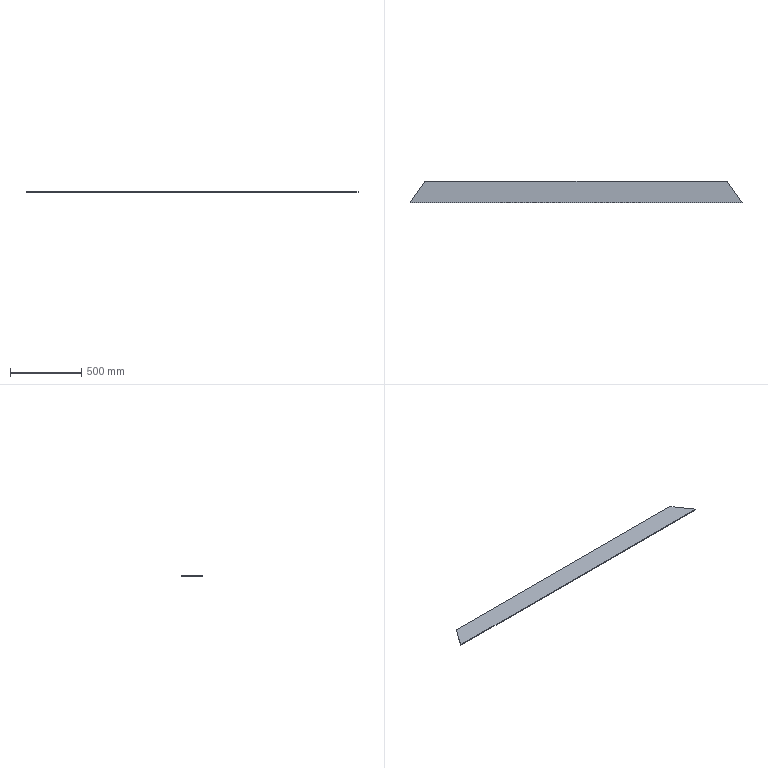Part | SolidWorks | features FlatPattern 1, SMBaseFlange 1, SheetMetal 1 | 1 solid | 6 faces | box 2328 x 150 x 6 mm | volume 2000672 mm3 | plane 6
STEP:
#1=CARTESIAN_POINT('',(105.031,150.,0.));
#2=VERTEX_POINT('',#1);
#3=CARTESIAN_POINT('',(0.,0.,0.));
#4=VERTEX_POINT('',#3);
#5=CARTESIAN_POINT('',(105.031,150.,0.));
#6=DIRECTION('',(-0.5736,-0.8192,0.));
#7=VECTOR('',#6,1000.);
#8=LINE('',#5,#7);
#9=EDGE_CURVE('',#2,#4,#8,.T.);
#10=ORIENTED_EDGE('',*,*,#9,.F.);
#11=CARTESIAN_POINT('',(105.031,150.,-6.));
#12=VERTEX_POINT('',#11);
#13=CARTESIAN_POINT('',(105.031,150.,-6.));
#14=DIRECTION('',(0.,0.,1.));
#15=VECTOR('',#14,1000.);
#16=LINE('',#13,#15);
#17=EDGE_CURVE('',#12,#2,#16,.T.);
#18=ORIENTED_EDGE('',*,*,#17,.F.);
#19=CARTESIAN_POINT('',(0.,0.,-6.));
#20=VERTEX_POINT('',#19);
#21=CARTESIAN_POINT('',(105.031,150.,-6.));
#22=DIRECTION('',(-0.5736,-0.8192,0.));
#23=VECTOR('',#22,1000.);
#24=LINE('',#21,#23);
#25=EDGE_CURVE('',#12,#20,#24,.T.);
#26=ORIENTED_EDGE('',*,*,#25,.T.);
#27=CARTESIAN_POINT('',(0.,0.,-6.));
#28=DIRECTION('',(0.,0.,1.));
#29=VECTOR('',#28,1000.);
#30=LINE('',#27,#29);
#31=EDGE_CURVE('',#20,#4,#30,.T.);
#32=ORIENTED_EDGE('',*,*,#31,.T.);
#33=EDGE_LOOP('',(#10,#18,#26,#32));
#34=FACE_OUTER_BOUND('',#33,.T.);
#35=CARTESIAN_POINT('',(105.031,150.,-6.));
#36=DIRECTION('',(-0.8192,0.5736,0.));
#37=DIRECTION('',(-0.5736,-0.8192,0.));
#38=AXIS2_PLACEMENT_3D('',#35,#36,#37);
#39=PLANE('',#38);
#40=ADVANCED_FACE('',(#34),#39,.T.);
#41=CARTESIAN_POINT('',(2222.969,150.,0.));
#42=VERTEX_POINT('',#41);
#43=CARTESIAN_POINT('',(2222.969,150.,0.));
#44=DIRECTION('',(-1.,0.,0.));
#45=VECTOR('',#44,1000.);
#46=LINE('',#43,#45);
#47=EDGE_CURVE('',#42,#2,#46,.T.);
#48=ORIENTED_EDGE('',*,*,#47,.F.);
#49=CARTESIAN_POINT('',(2222.969,150.,-6.));
#50=VERTEX_POINT('',#49);
#51=CARTESIAN_POINT('',(2222.969,150.,-6.));
#52=DIRECTION('',(0.,0.,1.));
#53=VECTOR('',#52,1000.);
#54=LINE('',#51,#53);
#55=EDGE_CURVE('',#50,#42,#54,.T.);
#56=ORIENTED_EDGE('',*,*,#55,.F.);
#57=CARTESIAN_POINT('',(2222.969,150.,-6.));
#58=DIRECTION('',(-1.,0.,0.));
#59=VECTOR('',#58,1000.);
#60=LINE('',#57,#59);
#61=EDGE_CURVE('',#50,#12,#60,.T.);
#62=ORIENTED_EDGE('',*,*,#61,.T.);
#63=ORIENTED_EDGE('',*,*,#17,.T.);
#64=EDGE_LOOP('',(#48,#56,#62,#63));
#65=FACE_OUTER_BOUND('',#64,.T.);
#66=CARTESIAN_POINT('',(2222.969,150.,-6.));
#67=DIRECTION('',(0.,1.,0.));
#68=DIRECTION('',(-1.,0.,0.));
#69=AXIS2_PLACEMENT_3D('',#66,#67,#68);
#70=PLANE('',#69);
#71=ADVANCED_FACE('',(#65),#70,.T.);
#72=CARTESIAN_POINT('',(2328.,0.,0.));
#73=VERTEX_POINT('',#72);
#74=CARTESIAN_POINT('',(2328.,0.,0.));
#75=DIRECTION('',(-0.5736,0.8192,0.));
#76=VECTOR('',#75,1000.);
#77=LINE('',#74,#76);
#78=EDGE_CURVE('',#73,#42,#77,.T.);
#79=ORIENTED_EDGE('',*,*,#78,.F.);
#80=CARTESIAN_POINT('',(2328.,0.,-6.));
#81=VERTEX_POINT('',#80);
#82=CARTESIAN_POINT('',(2328.,0.,-6.));
#83=DIRECTION('',(0.,0.,1.));
#84=VECTOR('',#83,1000.);
#85=LINE('',#82,#84);
#86=EDGE_CURVE('',#81,#73,#85,.T.);
#87=ORIENTED_EDGE('',*,*,#86,.F.);
#88=CARTESIAN_POINT('',(2328.,0.,-6.));
#89=DIRECTION('',(-0.5736,0.8192,0.));
#90=VECTOR('',#89,1000.);
#91=LINE('',#88,#90);
#92=EDGE_CURVE('',#81,#50,#91,.T.);
#93=ORIENTED_EDGE('',*,*,#92,.T.);
#94=ORIENTED_EDGE('',*,*,#55,.T.);
#95=EDGE_LOOP('',(#79,#87,#93,#94));
#96=FACE_OUTER_BOUND('',#95,.T.);
#97=CARTESIAN_POINT('',(2328.,0.,-6.));
#98=DIRECTION('',(0.8192,0.5736,0.));
#99=DIRECTION('',(-0.5736,0.8192,0.));
#100=AXIS2_PLACEMENT_3D('',#97,#98,#99);
#101=PLANE('',#100);
#102=ADVANCED_FACE('',(#96),#101,.T.);
#103=CARTESIAN_POINT('',(0.,0.,0.));
#104=DIRECTION('',(1.,0.,0.));
#105=VECTOR('',#104,1000.);
#106=LINE('',#103,#105);
#107=EDGE_CURVE('',#4,#73,#106,.T.);
#108=ORIENTED_EDGE('',*,*,#107,.F.);
#109=ORIENTED_EDGE('',*,*,#31,.F.);
#110=CARTESIAN_POINT('',(0.,0.,-6.));
#111=DIRECTION('',(1.,0.,0.));
#112=VECTOR('',#111,1000.);
#113=LINE('',#110,#112);
#114=EDGE_CURVE('',#20,#81,#113,.T.);
#115=ORIENTED_EDGE('',*,*,#114,.T.);
#116=ORIENTED_EDGE('',*,*,#86,.T.);
#117=EDGE_LOOP('',(#108,#109,#115,#116));
#118=FACE_OUTER_BOUND('',#117,.T.);
#119=CARTESIAN_POINT('',(0.,0.,-6.));
#120=DIRECTION('',(0.,-1.,0.));
#121=DIRECTION('',(0.,0.,-1.));
#122=AXIS2_PLACEMENT_3D('',#119,#120,#121);
#123=PLANE('',#122);
#124=ADVANCED_FACE('',(#118),#123,.T.);
#125=ORIENTED_EDGE('',*,*,#25,.F.);
#126=ORIENTED_EDGE('',*,*,#61,.F.);
#127=ORIENTED_EDGE('',*,*,#92,.F.);
#128=ORIENTED_EDGE('',*,*,#114,.F.);
#129=EDGE_LOOP('',(#125,#126,#127,#128));
#130=FACE_OUTER_BOUND('',#129,.T.);
#131=CARTESIAN_POINT('',(0.,0.,-6.));
#132=DIRECTION('',(0.,0.,-1.));
#133=DIRECTION('',(-1.,0.,0.));
#134=AXIS2_PLACEMENT_3D('',#131,#132,#133);
#135=PLANE('',#134);
#136=ADVANCED_FACE('',(#130),#135,.T.);
#137=ORIENTED_EDGE('',*,*,#9,.T.);
#138=ORIENTED_EDGE('',*,*,#107,.T.);
#139=ORIENTED_EDGE('',*,*,#78,.T.);
#140=ORIENTED_EDGE('',*,*,#47,.T.);
#141=EDGE_LOOP('',(#137,#138,#139,#140));
#142=FACE_OUTER_BOUND('',#141,.T.);
#143=CARTESIAN_POINT('',(0.,0.,0.));
#144=DIRECTION('',(0.,0.,-1.));
#145=DIRECTION('',(-1.,0.,0.));
#146=AXIS2_PLACEMENT_3D('',#143,#144,#145);
#147=PLANE('',#146);
#148=ADVANCED_FACE('',(#142),#147,.F.);
#149=CLOSED_SHELL('',(#40,#71,#102,#124,#136,#148));
#150=MANIFOLD_SOLID_BREP('',#149);
#151=CARTESIAN_POINT('',(0.,0.,0.));
#152=DIRECTION('',(0.,0.,1.));
#153=DIRECTION('',(1.,0.,0.));
#154=AXIS2_PLACEMENT_3D('',#151,#152,#153);
#155=(LENGTH_UNIT()NAMED_UNIT(*)SI_UNIT(.MILLI.,.METRE.));
#156=UNCERTAINTY_MEASURE_WITH_UNIT(LENGTH_MEASURE(0.00001),#155,'','');
#157=(NAMED_UNIT(*)PLANE_ANGLE_UNIT()SI_UNIT($,.RADIAN.));
#158=(NAMED_UNIT(*)SI_UNIT($,.STERADIAN.)SOLID_ANGLE_UNIT());
#159=(GEOMETRIC_REPRESENTATION_CONTEXT(3)GLOBAL_UNCERTAINTY_ASSIGNED_CONTEXT((#156))GLOBAL_UNIT_ASSIGNED_CONTEXT((#155,#157,#158))REPRESENTATION_CONTEXT('',''));
#160=ADVANCED_BREP_SHAPE_REPRESENTATION('',(#150,#154),#159);